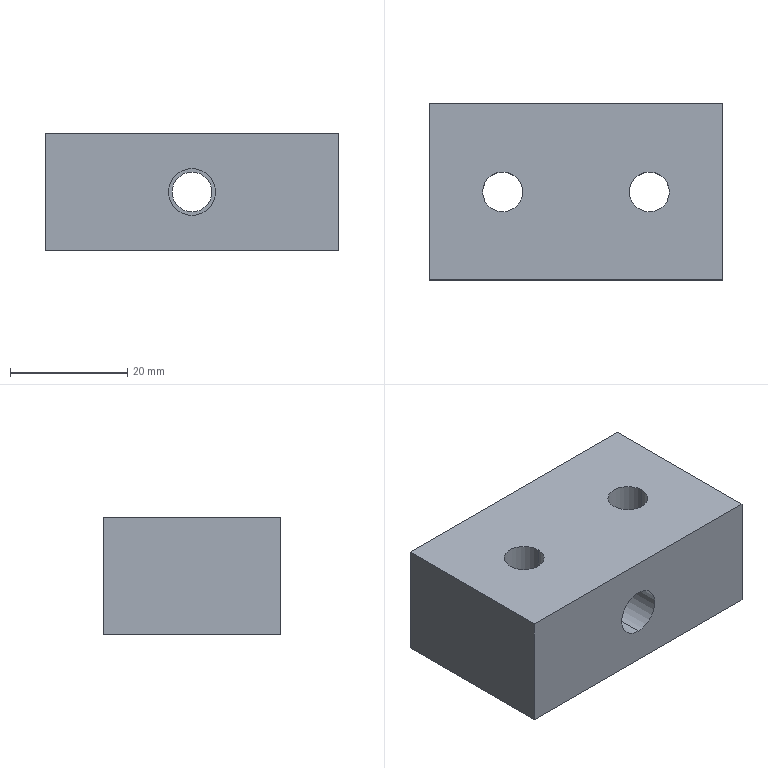Part | SolidWorks | features HoleWzd 2, 3DProfileFeature 1, Extrusion 1, ICE 1 | 1 solid | 15 faces | box 50 x 30 x 20 mm | volume 27179 mm3 | cylinder 8 | plane 7 | commonest cylinder face diameters 6.8 x6 8 x2
STEP:
#1=CARTESIAN_POINT('',(25.,-10.,14.));
#2=VERTEX_POINT('',#1);
#3=CARTESIAN_POINT('',(25.,-10.,6.));
#4=VERTEX_POINT('',#3);
#5=CARTESIAN_POINT('',(25.,-10.,10.));
#6=DIRECTION('',(0.,-1.,0.));
#7=DIRECTION('',(0.,0.,-1.));
#8=AXIS2_PLACEMENT_3D('',#5,#6,#7);
#9=CIRCLE('',#8,4.);
#10=EDGE_CURVE('',#2,#4,#9,.T.);
#11=ORIENTED_EDGE('',*,*,#10,.F.);
#12=CARTESIAN_POINT('',(25.,-30.,14.));
#13=VERTEX_POINT('',#12);
#14=CARTESIAN_POINT('',(25.,-10.,14.));
#15=DIRECTION('',(0.,-1.,0.));
#16=VECTOR('',#15,1000.);
#17=LINE('',#14,#16);
#18=EDGE_CURVE('',#2,#13,#17,.T.);
#19=ORIENTED_EDGE('',*,*,#18,.T.);
#20=CARTESIAN_POINT('',(25.,-30.,6.));
#21=VERTEX_POINT('',#20);
#22=CARTESIAN_POINT('',(25.,-30.,10.));
#23=DIRECTION('',(0.,-1.,0.));
#24=DIRECTION('',(0.,0.,-1.));
#25=AXIS2_PLACEMENT_3D('',#22,#23,#24);
#26=CIRCLE('',#25,4.);
#27=EDGE_CURVE('',#13,#21,#26,.T.);
#28=ORIENTED_EDGE('',*,*,#27,.T.);
#29=CARTESIAN_POINT('',(25.,-10.,6.));
#30=DIRECTION('',(0.,-1.,0.));
#31=VECTOR('',#30,1000.);
#32=LINE('',#29,#31);
#33=EDGE_CURVE('',#4,#21,#32,.T.);
#34=ORIENTED_EDGE('',*,*,#33,.F.);
#35=EDGE_LOOP('',(#11,#19,#28,#34));
#36=FACE_OUTER_BOUND('',#35,.T.);
#37=CARTESIAN_POINT('',(25.,-10.,10.));
#38=DIRECTION('',(0.,-1.,0.));
#39=DIRECTION('',(0.,0.,-1.));
#40=AXIS2_PLACEMENT_3D('',#37,#38,#39);
#41=CYLINDRICAL_SURFACE('',#40,4.);
#42=ADVANCED_FACE('',(#36),#41,.F.);
#43=CARTESIAN_POINT('',(40.9,-15.,20.));
#44=VERTEX_POINT('',#43);
#45=CARTESIAN_POINT('',(34.1,-15.,20.));
#46=VERTEX_POINT('',#45);
#47=CARTESIAN_POINT('',(37.5,-15.,20.));
#48=DIRECTION('',(0.,0.,-1.));
#49=DIRECTION('',(-1.,0.,0.));
#50=AXIS2_PLACEMENT_3D('',#47,#48,#49);
#51=CIRCLE('',#50,3.4);
#52=EDGE_CURVE('',#44,#46,#51,.T.);
#53=ORIENTED_EDGE('',*,*,#52,.F.);
#54=CARTESIAN_POINT('',(40.9,-15.,0.));
#55=VERTEX_POINT('',#54);
#56=CARTESIAN_POINT('',(40.9,-15.,0.));
#57=DIRECTION('',(0.,0.,-1.));
#58=VECTOR('',#57,1000.);
#59=LINE('',#56,#58);
#60=EDGE_CURVE('',#44,#55,#59,.T.);
#61=ORIENTED_EDGE('',*,*,#60,.T.);
#62=CARTESIAN_POINT('',(34.1,-15.,0.));
#63=VERTEX_POINT('',#62);
#64=CARTESIAN_POINT('',(37.5,-15.,0.));
#65=DIRECTION('',(0.,0.,-1.));
#66=DIRECTION('',(-1.,0.,0.));
#67=AXIS2_PLACEMENT_3D('',#64,#65,#66);
#68=CIRCLE('',#67,3.4);
#69=EDGE_CURVE('',#55,#63,#68,.T.);
#70=ORIENTED_EDGE('',*,*,#69,.T.);
#71=CARTESIAN_POINT('',(34.1,-15.,0.));
#72=DIRECTION('',(0.,0.,-1.));
#73=VECTOR('',#72,1000.);
#74=LINE('',#71,#73);
#75=EDGE_CURVE('',#46,#63,#74,.T.);
#76=ORIENTED_EDGE('',*,*,#75,.F.);
#77=EDGE_LOOP('',(#53,#61,#70,#76));
#78=FACE_OUTER_BOUND('',#77,.T.);
#79=CARTESIAN_POINT('',(37.5,-15.,0.));
#80=DIRECTION('',(0.,0.,-1.));
#81=DIRECTION('',(-1.,0.,0.));
#82=AXIS2_PLACEMENT_3D('',#79,#80,#81);
#83=CYLINDRICAL_SURFACE('',#82,3.4);
#84=ADVANCED_FACE('',(#78),#83,.F.);
#85=CARTESIAN_POINT('',(15.9,-15.,20.));
#86=VERTEX_POINT('',#85);
#87=CARTESIAN_POINT('',(9.1,-15.,20.));
#88=VERTEX_POINT('',#87);
#89=CARTESIAN_POINT('',(12.5,-15.,20.));
#90=DIRECTION('',(0.,0.,-1.));
#91=DIRECTION('',(-1.,0.,0.));
#92=AXIS2_PLACEMENT_3D('',#89,#90,#91);
#93=CIRCLE('',#92,3.4);
#94=EDGE_CURVE('',#86,#88,#93,.T.);
#95=ORIENTED_EDGE('',*,*,#94,.F.);
#96=CARTESIAN_POINT('',(15.9,-15.,0.));
#97=VERTEX_POINT('',#96);
#98=CARTESIAN_POINT('',(15.9,-15.,0.));
#99=DIRECTION('',(0.,0.,-1.));
#100=VECTOR('',#99,1000.);
#101=LINE('',#98,#100);
#102=EDGE_CURVE('',#86,#97,#101,.T.);
#103=ORIENTED_EDGE('',*,*,#102,.T.);
#104=CARTESIAN_POINT('',(9.1,-15.,0.));
#105=VERTEX_POINT('',#104);
#106=CARTESIAN_POINT('',(12.5,-15.,0.));
#107=DIRECTION('',(0.,0.,-1.));
#108=DIRECTION('',(-1.,0.,0.));
#109=AXIS2_PLACEMENT_3D('',#106,#107,#108);
#110=CIRCLE('',#109,3.4);
#111=EDGE_CURVE('',#97,#105,#110,.T.);
#112=ORIENTED_EDGE('',*,*,#111,.T.);
#113=CARTESIAN_POINT('',(9.1,-15.,0.));
#114=DIRECTION('',(0.,0.,-1.));
#115=VECTOR('',#114,1000.);
#116=LINE('',#113,#115);
#117=EDGE_CURVE('',#88,#105,#116,.T.);
#118=ORIENTED_EDGE('',*,*,#117,.F.);
#119=EDGE_LOOP('',(#95,#103,#112,#118));
#120=FACE_OUTER_BOUND('',#119,.T.);
#121=CARTESIAN_POINT('',(12.5,-15.,0.));
#122=DIRECTION('',(0.,0.,-1.));
#123=DIRECTION('',(-1.,0.,0.));
#124=AXIS2_PLACEMENT_3D('',#121,#122,#123);
#125=CYLINDRICAL_SURFACE('',#124,3.4);
#126=ADVANCED_FACE('',(#120),#125,.F.);
#127=CARTESIAN_POINT('',(25.,-10.,6.6));
#128=VERTEX_POINT('',#127);
#129=CARTESIAN_POINT('',(25.,-10.,13.4));
#130=VERTEX_POINT('',#129);
#131=CARTESIAN_POINT('',(25.,-10.,10.));
#132=DIRECTION('',(0.,1.,0.));
#133=DIRECTION('',(0.,0.,-1.));
#134=AXIS2_PLACEMENT_3D('',#131,#132,#133);
#135=CIRCLE('',#134,3.4);
#136=EDGE_CURVE('',#128,#130,#135,.T.);
#137=ORIENTED_EDGE('',*,*,#136,.F.);
#138=CARTESIAN_POINT('',(25.,0.,6.6));
#139=VERTEX_POINT('',#138);
#140=CARTESIAN_POINT('',(25.,0.,6.6));
#141=DIRECTION('',(0.,1.,0.));
#142=VECTOR('',#141,1000.);
#143=LINE('',#140,#142);
#144=EDGE_CURVE('',#128,#139,#143,.T.);
#145=ORIENTED_EDGE('',*,*,#144,.T.);
#146=CARTESIAN_POINT('',(25.,0.,13.4));
#147=VERTEX_POINT('',#146);
#148=CARTESIAN_POINT('',(25.,0.,10.));
#149=DIRECTION('',(0.,1.,0.));
#150=DIRECTION('',(0.,0.,1.));
#151=AXIS2_PLACEMENT_3D('',#148,#149,#150);
#152=CIRCLE('',#151,3.4);
#153=EDGE_CURVE('',#139,#147,#152,.T.);
#154=ORIENTED_EDGE('',*,*,#153,.T.);
#155=CARTESIAN_POINT('',(25.,0.,13.4));
#156=DIRECTION('',(0.,1.,0.));
#157=VECTOR('',#156,1000.);
#158=LINE('',#155,#157);
#159=EDGE_CURVE('',#130,#147,#158,.T.);
#160=ORIENTED_EDGE('',*,*,#159,.F.);
#161=EDGE_LOOP('',(#137,#145,#154,#160));
#162=FACE_OUTER_BOUND('',#161,.T.);
#163=CARTESIAN_POINT('',(25.,0.,10.));
#164=DIRECTION('',(0.,1.,0.));
#165=DIRECTION('',(0.,0.,1.));
#166=AXIS2_PLACEMENT_3D('',#163,#164,#165);
#167=CYLINDRICAL_SURFACE('',#166,3.4);
#168=ADVANCED_FACE('',(#162),#167,.F.);
#169=ORIENTED_EDGE('',*,*,#144,.F.);
#170=CARTESIAN_POINT('',(25.,-10.,10.));
#171=DIRECTION('',(0.,1.,0.));
#172=DIRECTION('',(0.,0.,-1.));
#173=AXIS2_PLACEMENT_3D('',#170,#171,#172);
#174=CIRCLE('',#173,3.4);
#175=EDGE_CURVE('',#130,#128,#174,.T.);
#176=ORIENTED_EDGE('',*,*,#175,.F.);
#177=ORIENTED_EDGE('',*,*,#159,.T.);
#178=CARTESIAN_POINT('',(25.,0.,10.));
#179=DIRECTION('',(0.,1.,0.));
#180=DIRECTION('',(0.,0.,1.));
#181=AXIS2_PLACEMENT_3D('',#178,#179,#180);
#182=CIRCLE('',#181,3.4);
#183=EDGE_CURVE('',#147,#139,#182,.T.);
#184=ORIENTED_EDGE('',*,*,#183,.T.);
#185=EDGE_LOOP('',(#169,#176,#177,#184));
#186=FACE_OUTER_BOUND('',#185,.T.);
#187=CARTESIAN_POINT('',(25.,0.,10.));
#188=DIRECTION('',(0.,1.,0.));
#189=DIRECTION('',(0.,0.,1.));
#190=AXIS2_PLACEMENT_3D('',#187,#188,#189);
#191=CYLINDRICAL_SURFACE('',#190,3.4);
#192=ADVANCED_FACE('',(#186),#191,.F.);
#193=CARTESIAN_POINT('',(0.,0.,0.));
#194=VERTEX_POINT('',#193);
#195=CARTESIAN_POINT('',(0.,-30.,0.));
#196=VERTEX_POINT('',#195);
#197=CARTESIAN_POINT('',(0.,0.,0.));
#198=DIRECTION('',(0.,-1.,0.));
#199=VECTOR('',#198,1000.);
#200=LINE('',#197,#199);
#201=EDGE_CURVE('',#194,#196,#200,.T.);
#202=ORIENTED_EDGE('',*,*,#201,.T.);
#203=CARTESIAN_POINT('',(0.,-30.,20.));
#204=VERTEX_POINT('',#203);
#205=CARTESIAN_POINT('',(0.,-30.,20.));
#206=DIRECTION('',(0.,0.,-1.));
#207=VECTOR('',#206,1000.);
#208=LINE('',#205,#207);
#209=EDGE_CURVE('',#204,#196,#208,.T.);
#210=ORIENTED_EDGE('',*,*,#209,.F.);
#211=CARTESIAN_POINT('',(0.,0.,20.));
#212=VERTEX_POINT('',#211);
#213=CARTESIAN_POINT('',(0.,0.,20.));
#214=DIRECTION('',(0.,-1.,0.));
#215=VECTOR('',#214,1000.);
#216=LINE('',#213,#215);
#217=EDGE_CURVE('',#212,#204,#216,.T.);
#218=ORIENTED_EDGE('',*,*,#217,.F.);
#219=CARTESIAN_POINT('',(0.,0.,20.));
#220=DIRECTION('',(0.,0.,-1.));
#221=VECTOR('',#220,1000.);
#222=LINE('',#219,#221);
#223=EDGE_CURVE('',#212,#194,#222,.T.);
#224=ORIENTED_EDGE('',*,*,#223,.T.);
#225=EDGE_LOOP('',(#202,#210,#218,#224));
#226=FACE_OUTER_BOUND('',#225,.T.);
#227=CARTESIAN_POINT('',(0.,0.,20.));
#228=DIRECTION('',(1.,0.,0.));
#229=DIRECTION('',(0.,1.,0.));
#230=AXIS2_PLACEMENT_3D('',#227,#228,#229);
#231=PLANE('',#230);
#232=ADVANCED_FACE('',(#226),#231,.F.);
#233=CARTESIAN_POINT('',(25.,-30.,10.));
#234=DIRECTION('',(0.,-1.,0.));
#235=DIRECTION('',(0.,0.,-1.));
#236=AXIS2_PLACEMENT_3D('',#233,#234,#235);
#237=CIRCLE('',#236,4.);
#238=EDGE_CURVE('',#21,#13,#237,.T.);
#239=ORIENTED_EDGE('',*,*,#238,.F.);
#240=ORIENTED_EDGE('',*,*,#27,.F.);
#241=EDGE_LOOP('',(#239,#240));
#242=FACE_BOUND('',#241,.T.);
#243=CARTESIAN_POINT('',(50.,-30.,0.));
#244=VERTEX_POINT('',#243);
#245=CARTESIAN_POINT('',(0.,-30.,0.));
#246=DIRECTION('',(1.,0.,0.));
#247=VECTOR('',#246,1000.);
#248=LINE('',#245,#247);
#249=EDGE_CURVE('',#196,#244,#248,.T.);
#250=ORIENTED_EDGE('',*,*,#249,.T.);
#251=CARTESIAN_POINT('',(50.,-30.,20.));
#252=VERTEX_POINT('',#251);
#253=CARTESIAN_POINT('',(50.,-30.,20.));
#254=DIRECTION('',(0.,0.,-1.));
#255=VECTOR('',#254,1000.);
#256=LINE('',#253,#255);
#257=EDGE_CURVE('',#252,#244,#256,.T.);
#258=ORIENTED_EDGE('',*,*,#257,.F.);
#259=CARTESIAN_POINT('',(0.,-30.,20.));
#260=DIRECTION('',(1.,0.,0.));
#261=VECTOR('',#260,1000.);
#262=LINE('',#259,#261);
#263=EDGE_CURVE('',#204,#252,#262,.T.);
#264=ORIENTED_EDGE('',*,*,#263,.F.);
#265=ORIENTED_EDGE('',*,*,#209,.T.);
#266=EDGE_LOOP('',(#250,#258,#264,#265));
#267=FACE_OUTER_BOUND('',#266,.T.);
#268=CARTESIAN_POINT('',(0.,-30.,20.));
#269=DIRECTION('',(0.,1.,0.));
#270=DIRECTION('',(0.,0.,1.));
#271=AXIS2_PLACEMENT_3D('',#268,#269,#270);
#272=PLANE('',#271);
#273=ADVANCED_FACE('',(#242,#267),#272,.F.);
#274=CARTESIAN_POINT('',(50.,0.,0.));
#275=VERTEX_POINT('',#274);
#276=CARTESIAN_POINT('',(50.,0.,0.));
#277=DIRECTION('',(0.,1.,0.));
#278=VECTOR('',#277,1000.);
#279=LINE('',#276,#278);
#280=EDGE_CURVE('',#244,#275,#279,.T.);
#281=ORIENTED_EDGE('',*,*,#280,.T.);
#282=CARTESIAN_POINT('',(50.,0.,20.));
#283=VERTEX_POINT('',#282);
#284=CARTESIAN_POINT('',(50.,0.,20.));
#285=DIRECTION('',(0.,0.,-1.));
#286=VECTOR('',#285,1000.);
#287=LINE('',#284,#286);
#288=EDGE_CURVE('',#283,#275,#287,.T.);
#289=ORIENTED_EDGE('',*,*,#288,.F.);
#290=CARTESIAN_POINT('',(50.,0.,20.));
#291=DIRECTION('',(0.,1.,0.));
#292=VECTOR('',#291,1000.);
#293=LINE('',#290,#292);
#294=EDGE_CURVE('',#252,#283,#293,.T.);
#295=ORIENTED_EDGE('',*,*,#294,.F.);
#296=ORIENTED_EDGE('',*,*,#257,.T.);
#297=EDGE_LOOP('',(#281,#289,#295,#296));
#298=FACE_OUTER_BOUND('',#297,.T.);
#299=CARTESIAN_POINT('',(50.,0.,20.));
#300=DIRECTION('',(-1.,0.,0.));
#301=DIRECTION('',(0.,-1.,0.));
#302=AXIS2_PLACEMENT_3D('',#299,#300,#301);
#303=PLANE('',#302);
#304=ADVANCED_FACE('',(#298),#303,.F.);
#305=ORIENTED_EDGE('',*,*,#183,.F.);
#306=ORIENTED_EDGE('',*,*,#153,.F.);
#307=EDGE_LOOP('',(#305,#306));
#308=FACE_BOUND('',#307,.T.);
#309=CARTESIAN_POINT('',(0.,0.,0.));
#310=DIRECTION('',(-1.,0.,0.));
#311=VECTOR('',#310,1000.);
#312=LINE('',#309,#311);
#313=EDGE_CURVE('',#275,#194,#312,.T.);
#314=ORIENTED_EDGE('',*,*,#313,.T.);
#315=ORIENTED_EDGE('',*,*,#223,.F.);
#316=CARTESIAN_POINT('',(0.,0.,20.));
#317=DIRECTION('',(-1.,0.,0.));
#318=VECTOR('',#317,1000.);
#319=LINE('',#316,#318);
#320=EDGE_CURVE('',#283,#212,#319,.T.);
#321=ORIENTED_EDGE('',*,*,#320,.F.);
#322=ORIENTED_EDGE('',*,*,#288,.T.);
#323=EDGE_LOOP('',(#314,#315,#321,#322));
#324=FACE_OUTER_BOUND('',#323,.T.);
#325=CARTESIAN_POINT('',(0.,0.,20.));
#326=DIRECTION('',(0.,-1.,0.));
#327=DIRECTION('',(0.,0.,-1.));
#328=AXIS2_PLACEMENT_3D('',#325,#326,#327);
#329=PLANE('',#328);
#330=ADVANCED_FACE('',(#308,#324),#329,.F.);
#331=CARTESIAN_POINT('',(37.5,-15.,20.));
#332=DIRECTION('',(0.,0.,-1.));
#333=DIRECTION('',(-1.,0.,0.));
#334=AXIS2_PLACEMENT_3D('',#331,#332,#333);
#335=CIRCLE('',#334,3.4);
#336=EDGE_CURVE('',#46,#44,#335,.T.);
#337=ORIENTED_EDGE('',*,*,#336,.T.);
#338=ORIENTED_EDGE('',*,*,#52,.T.);
#339=EDGE_LOOP('',(#337,#338));
#340=FACE_BOUND('',#339,.T.);
#341=CARTESIAN_POINT('',(12.5,-15.,20.));
#342=DIRECTION('',(0.,0.,-1.));
#343=DIRECTION('',(-1.,0.,0.));
#344=AXIS2_PLACEMENT_3D('',#341,#342,#343);
#345=CIRCLE('',#344,3.4);
#346=EDGE_CURVE('',#88,#86,#345,.T.);
#347=ORIENTED_EDGE('',*,*,#346,.T.);
#348=ORIENTED_EDGE('',*,*,#94,.T.);
#349=EDGE_LOOP('',(#347,#348));
#350=FACE_BOUND('',#349,.T.);
#351=ORIENTED_EDGE('',*,*,#217,.T.);
#352=ORIENTED_EDGE('',*,*,#263,.T.);
#353=ORIENTED_EDGE('',*,*,#294,.T.);
#354=ORIENTED_EDGE('',*,*,#320,.T.);
#355=EDGE_LOOP('',(#351,#352,#353,#354));
#356=FACE_OUTER_BOUND('',#355,.T.);
#357=CARTESIAN_POINT('',(0.,0.,20.));
#358=DIRECTION('',(0.,0.,1.));
#359=DIRECTION('',(1.,0.,0.));
#360=AXIS2_PLACEMENT_3D('',#357,#358,#359);
#361=PLANE('',#360);
#362=ADVANCED_FACE('',(#340,#350,#356),#361,.T.);
#363=CARTESIAN_POINT('',(37.5,-15.,0.));
#364=DIRECTION('',(0.,0.,-1.));
#365=DIRECTION('',(-1.,0.,0.));
#366=AXIS2_PLACEMENT_3D('',#363,#364,#365);
#367=CIRCLE('',#366,3.4);
#368=EDGE_CURVE('',#63,#55,#367,.T.);
#369=ORIENTED_EDGE('',*,*,#368,.F.);
#370=ORIENTED_EDGE('',*,*,#69,.F.);
#371=EDGE_LOOP('',(#369,#370));
#372=FACE_BOUND('',#371,.T.);
#373=CARTESIAN_POINT('',(12.5,-15.,0.));
#374=DIRECTION('',(0.,0.,-1.));
#375=DIRECTION('',(-1.,0.,0.));
#376=AXIS2_PLACEMENT_3D('',#373,#374,#375);
#377=CIRCLE('',#376,3.4);
#378=EDGE_CURVE('',#105,#97,#377,.T.);
#379=ORIENTED_EDGE('',*,*,#378,.F.);
#380=ORIENTED_EDGE('',*,*,#111,.F.);
#381=EDGE_LOOP('',(#379,#380));
#382=FACE_BOUND('',#381,.T.);
#383=ORIENTED_EDGE('',*,*,#201,.F.);
#384=ORIENTED_EDGE('',*,*,#313,.F.);
#385=ORIENTED_EDGE('',*,*,#280,.F.);
#386=ORIENTED_EDGE('',*,*,#249,.F.);
#387=EDGE_LOOP('',(#383,#384,#385,#386));
#388=FACE_OUTER_BOUND('',#387,.T.);
#389=CARTESIAN_POINT('',(0.,0.,0.));
#390=DIRECTION('',(0.,0.,1.));
#391=DIRECTION('',(1.,0.,0.));
#392=AXIS2_PLACEMENT_3D('',#389,#390,#391);
#393=PLANE('',#392);
#394=ADVANCED_FACE('',(#372,#382,#388),#393,.F.);
#395=ORIENTED_EDGE('',*,*,#102,.F.);
#396=ORIENTED_EDGE('',*,*,#346,.F.);
#397=ORIENTED_EDGE('',*,*,#117,.T.);
#398=ORIENTED_EDGE('',*,*,#378,.T.);
#399=EDGE_LOOP('',(#395,#396,#397,#398));
#400=FACE_OUTER_BOUND('',#399,.T.);
#401=CARTESIAN_POINT('',(12.5,-15.,0.));
#402=DIRECTION('',(0.,0.,-1.));
#403=DIRECTION('',(-1.,0.,0.));
#404=AXIS2_PLACEMENT_3D('',#401,#402,#403);
#405=CYLINDRICAL_SURFACE('',#404,3.4);
#406=ADVANCED_FACE('',(#400),#405,.F.);
#407=ORIENTED_EDGE('',*,*,#60,.F.);
#408=ORIENTED_EDGE('',*,*,#336,.F.);
#409=ORIENTED_EDGE('',*,*,#75,.T.);
#410=ORIENTED_EDGE('',*,*,#368,.T.);
#411=EDGE_LOOP('',(#407,#408,#409,#410));
#412=FACE_OUTER_BOUND('',#411,.T.);
#413=CARTESIAN_POINT('',(37.5,-15.,0.));
#414=DIRECTION('',(0.,0.,-1.));
#415=DIRECTION('',(-1.,0.,0.));
#416=AXIS2_PLACEMENT_3D('',#413,#414,#415);
#417=CYLINDRICAL_SURFACE('',#416,3.4);
#418=ADVANCED_FACE('',(#412),#417,.F.);
#419=CARTESIAN_POINT('',(25.,-10.,10.));
#420=DIRECTION('',(0.,-1.,0.));
#421=DIRECTION('',(0.,0.,-1.));
#422=AXIS2_PLACEMENT_3D('',#419,#420,#421);
#423=CIRCLE('',#422,4.);
#424=EDGE_CURVE('',#4,#2,#423,.T.);
#425=ORIENTED_EDGE('',*,*,#424,.T.);
#426=ORIENTED_EDGE('',*,*,#10,.T.);
#427=EDGE_LOOP('',(#425,#426));
#428=FACE_OUTER_BOUND('',#427,.T.);
#429=ORIENTED_EDGE('',*,*,#175,.T.);
#430=ORIENTED_EDGE('',*,*,#136,.T.);
#431=EDGE_LOOP('',(#429,#430));
#432=FACE_BOUND('',#431,.T.);
#433=CARTESIAN_POINT('',(25.,-10.,10.));
#434=DIRECTION('',(0.,-1.,0.));
#435=DIRECTION('',(0.,0.,-1.));
#436=AXIS2_PLACEMENT_3D('',#433,#434,#435);
#437=PLANE('',#436);
#438=ADVANCED_FACE('',(#428,#432),#437,.T.);
#439=ORIENTED_EDGE('',*,*,#18,.F.);
#440=ORIENTED_EDGE('',*,*,#424,.F.);
#441=ORIENTED_EDGE('',*,*,#33,.T.);
#442=ORIENTED_EDGE('',*,*,#238,.T.);
#443=EDGE_LOOP('',(#439,#440,#441,#442));
#444=FACE_OUTER_BOUND('',#443,.T.);
#445=CARTESIAN_POINT('',(25.,-10.,10.));
#446=DIRECTION('',(0.,-1.,0.));
#447=DIRECTION('',(0.,0.,-1.));
#448=AXIS2_PLACEMENT_3D('',#445,#446,#447);
#449=CYLINDRICAL_SURFACE('',#448,4.);
#450=ADVANCED_FACE('',(#444),#449,.F.);
#451=CLOSED_SHELL('',(#42,#84,#126,#168,#192,#232,#273,#304,#330,#362,#394,#406,#418,#438,#450));
#452=MANIFOLD_SOLID_BREP('',#451);
#453=CARTESIAN_POINT('',(0.,0.,0.));
#454=DIRECTION('',(0.,0.,1.));
#455=DIRECTION('',(1.,0.,0.));
#456=AXIS2_PLACEMENT_3D('',#453,#454,#455);
#457=(LENGTH_UNIT()NAMED_UNIT(*)SI_UNIT(.MILLI.,.METRE.));
#458=UNCERTAINTY_MEASURE_WITH_UNIT(LENGTH_MEASURE(0.00001),#457,'','');
#459=(NAMED_UNIT(*)PLANE_ANGLE_UNIT()SI_UNIT($,.RADIAN.));
#460=(NAMED_UNIT(*)SI_UNIT($,.STERADIAN.)SOLID_ANGLE_UNIT());
#461=(GEOMETRIC_REPRESENTATION_CONTEXT(3)GLOBAL_UNCERTAINTY_ASSIGNED_CONTEXT((#458))GLOBAL_UNIT_ASSIGNED_CONTEXT((#457,#459,#460))REPRESENTATION_CONTEXT('',''));
#462=ADVANCED_BREP_SHAPE_REPRESENTATION('',(#452,#456),#461);